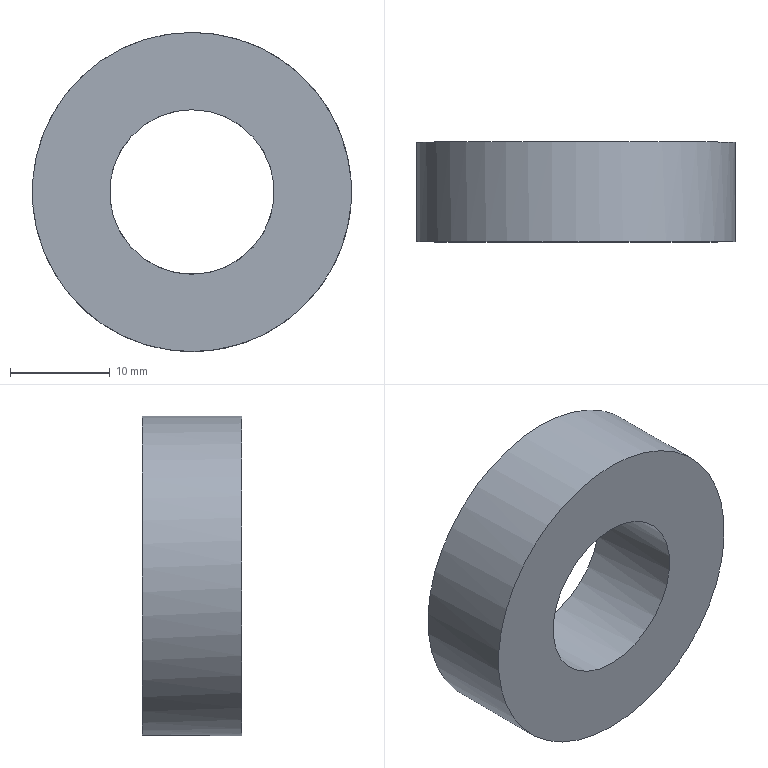Part | NX | features solid 2 | 1 solid | 4 faces | box 32 x 10 x 32 mm | volume 5904 mm3 | cylinder 2 | plane 2 | commonest cylinder face diameters 16.5 x1 32 x1
STEP:
#1=CARTESIAN_POINT('',(-280.,540.,-371.75));
#2=VERTEX_POINT('',#1);
#3=CARTESIAN_POINT('',(-280.,540.,-380.));
#4=DIRECTION('',(0.,-1.,0.));
#5=DIRECTION('',(0.,0.,1.));
#6=AXIS2_PLACEMENT_3D('',#3,#4,#5);
#7=CIRCLE('',#6,8.25);
#8=EDGE_CURVE('',#2,#2,#7,.T.);
#9=ORIENTED_EDGE('',*,*,#8,.T.);
#10=EDGE_LOOP('',(#9));
#11=FACE_BOUND('',#10,.T.);
#12=CARTESIAN_POINT('',(-271.75,550.,-380.));
#13=VERTEX_POINT('',#12);
#14=CARTESIAN_POINT('',(-280.,550.,-380.));
#15=DIRECTION('',(0.,-1.,0.));
#16=DIRECTION('',(1.,0.,0.));
#17=AXIS2_PLACEMENT_3D('',#14,#15,#16);
#18=CIRCLE('',#17,8.25);
#19=EDGE_CURVE('',#13,#13,#18,.T.);
#20=ORIENTED_EDGE('',*,*,#19,.F.);
#21=EDGE_LOOP('',(#20));
#22=FACE_BOUND('',#21,.T.);
#23=CARTESIAN_POINT('',(-280.,542.,-380.));
#24=DIRECTION('',(0.,1.,0.));
#25=DIRECTION('',(-1.,0.,0.));
#26=AXIS2_PLACEMENT_3D('',#23,#24,#25);
#27=CYLINDRICAL_SURFACE('',#26,8.25);
#28=ADVANCED_FACE('',(#11,#22),#27,.F.);
#29=CARTESIAN_POINT('',(-280.,540.,-364.));
#30=VERTEX_POINT('',#29);
#31=CARTESIAN_POINT('',(-280.,540.,-380.));
#32=DIRECTION('',(0.,-1.,0.));
#33=DIRECTION('',(0.,0.,1.));
#34=AXIS2_PLACEMENT_3D('',#31,#32,#33);
#35=CIRCLE('',#34,16.);
#36=EDGE_CURVE('',#30,#30,#35,.T.);
#37=ORIENTED_EDGE('',*,*,#36,.F.);
#38=EDGE_LOOP('',(#37));
#39=FACE_BOUND('',#38,.T.);
#40=CARTESIAN_POINT('',(-264.,550.,-380.));
#41=VERTEX_POINT('',#40);
#42=CARTESIAN_POINT('',(-280.,550.,-380.));
#43=DIRECTION('',(0.,-1.,0.));
#44=DIRECTION('',(1.,0.,0.));
#45=AXIS2_PLACEMENT_3D('',#42,#43,#44);
#46=CIRCLE('',#45,16.);
#47=EDGE_CURVE('',#41,#41,#46,.T.);
#48=ORIENTED_EDGE('',*,*,#47,.T.);
#49=EDGE_LOOP('',(#48));
#50=FACE_BOUND('',#49,.T.);
#51=CARTESIAN_POINT('',(-280.,542.,-380.));
#52=DIRECTION('',(0.,1.,0.));
#53=DIRECTION('',(-1.,0.,0.));
#54=AXIS2_PLACEMENT_3D('',#51,#52,#53);
#55=CYLINDRICAL_SURFACE('',#54,16.);
#56=ADVANCED_FACE('',(#39,#50),#55,.T.);
#57=ORIENTED_EDGE('',*,*,#8,.F.);
#58=EDGE_LOOP('',(#57));
#59=FACE_BOUND('',#58,.T.);
#60=ORIENTED_EDGE('',*,*,#36,.T.);
#61=EDGE_LOOP('',(#60));
#62=FACE_BOUND('',#61,.T.);
#63=CARTESIAN_POINT('',(-280.,540.,-380.));
#64=DIRECTION('',(0.,-1.,0.));
#65=DIRECTION('',(1.,0.,0.));
#66=AXIS2_PLACEMENT_3D('',#63,#64,#65);
#67=PLANE('',#66);
#68=ADVANCED_FACE('',(#59,#62),#67,.T.);
#69=ORIENTED_EDGE('',*,*,#19,.T.);
#70=EDGE_LOOP('',(#69));
#71=FACE_BOUND('',#70,.T.);
#72=ORIENTED_EDGE('',*,*,#47,.F.);
#73=EDGE_LOOP('',(#72));
#74=FACE_BOUND('',#73,.T.);
#75=CARTESIAN_POINT('',(-280.,550.,-380.));
#76=DIRECTION('',(0.,-1.,0.));
#77=DIRECTION('',(1.,0.,0.));
#78=AXIS2_PLACEMENT_3D('',#75,#76,#77);
#79=PLANE('',#78);
#80=ADVANCED_FACE('',(#71,#74),#79,.F.);
#81=CLOSED_SHELL('',(#28,#56,#68,#80));
#82=MANIFOLD_SOLID_BREP('',#81);
#83=(LENGTH_UNIT()NAMED_UNIT(*)SI_UNIT(.MILLI.,.METRE.));
#84=UNCERTAINTY_MEASURE_WITH_UNIT(LENGTH_MEASURE(0.00001),#83,'','');
#85=(NAMED_UNIT(*)PLANE_ANGLE_UNIT()SI_UNIT($,.RADIAN.));
#86=(NAMED_UNIT(*)SI_UNIT($,.STERADIAN.)SOLID_ANGLE_UNIT());
#87=(GEOMETRIC_REPRESENTATION_CONTEXT(3)GLOBAL_UNCERTAINTY_ASSIGNED_CONTEXT((#84))GLOBAL_UNIT_ASSIGNED_CONTEXT((#83,#85,#86))REPRESENTATION_CONTEXT('',''));
#88=ADVANCED_BREP_SHAPE_REPRESENTATION('',(#82),#87);